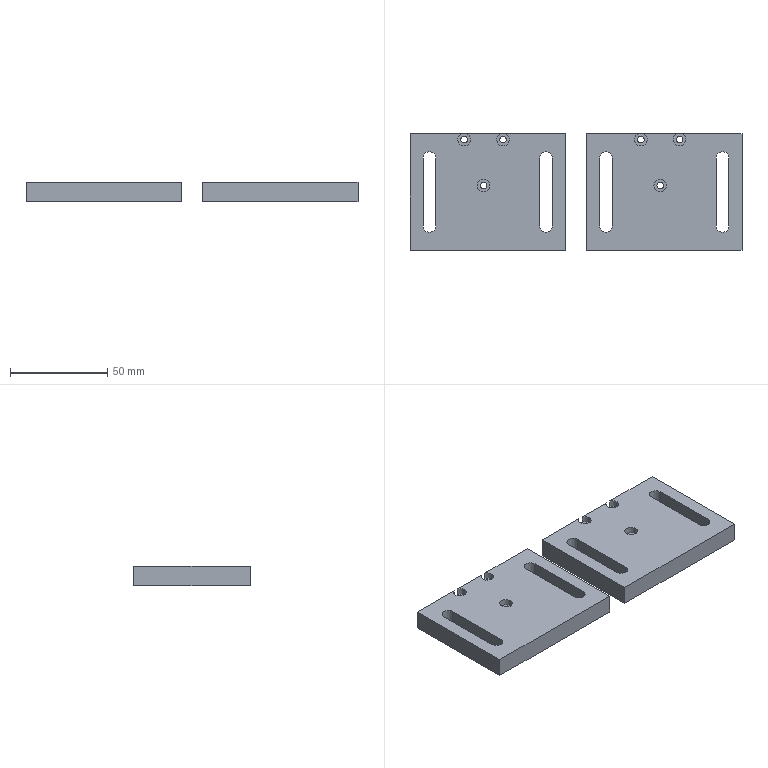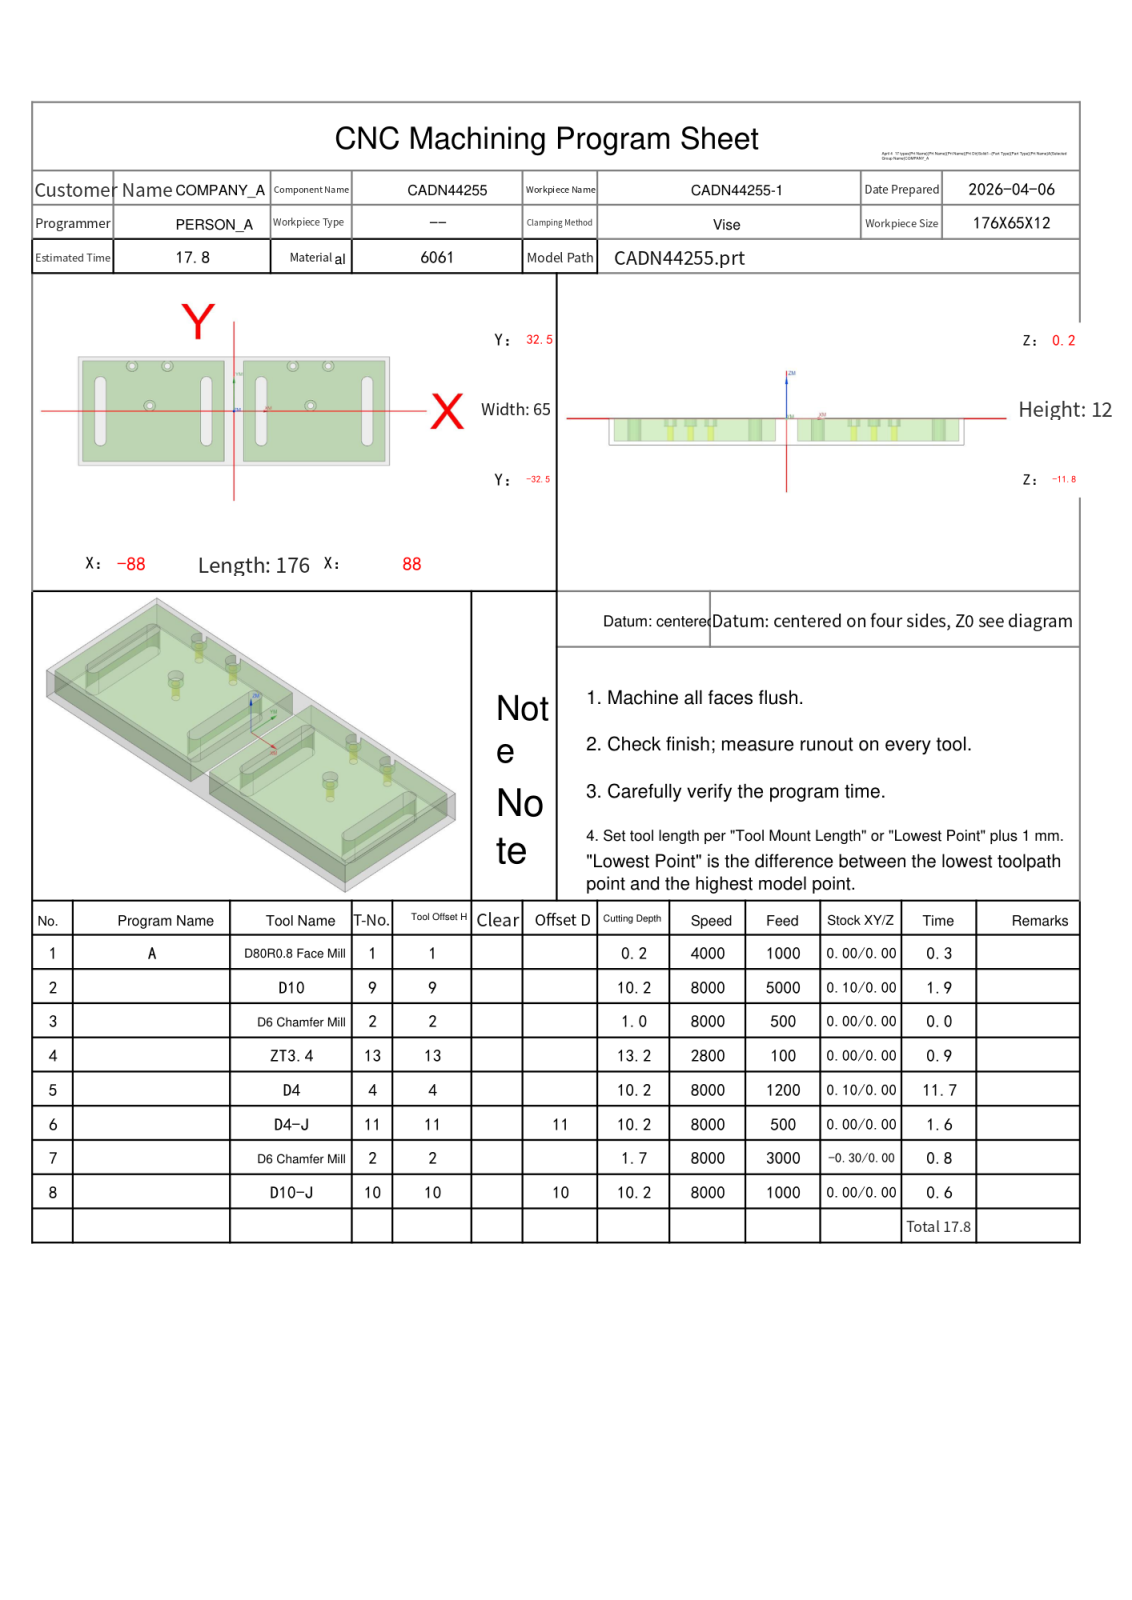NC program | NX | posted by the shop | part box 171 x 60 x 10 mm
Lines 1 to 1630 of 2411, first 1199 of 1628 lines:
%
O0001
(Machine time: 19.33 MIN)
(===Total Tool:7===)
(T1=D80R0.8 Face Mill D=80.  R=0.8  D-  H01 Z=0.    )
(T9=D10     D=10.  R=0.   D-  H09 Z=-10.  )
(T2=D6 Chamfer Mill  D=6.  R=0.  D-  H02 Z=-1.5  )
(T13=ZT3.4  D=3.4  DR_a=118 D-  H13 Z=-13.02)
(T4=D4      D=4.   R=0.   D-  H04 Z=-10.  )
(T11=D4-J   D=4.   R=0.   D11 H11 Z=-10.  )
(T10=D10-J  D=10.  R=0.   D10 H10 Z=-10.  )
G80 G90 G17 G49 G40
G91 G28 Z0
M01
N1 T01 M06
(D80R0.8 Face Mill  D=80. R=0.8 H=01 ce=0.00 di=0.00)
G00 G90 G54 X-130.5 Y0.0 M03 S4000
G43 H01 Z20.
M08
Z2.
G01 Z0.0 F1000.
X-125.5
X125.5
X130.5
Z2.
G00 Z20.
G91 G28 Z0.0
M05
M09
G91 G28 Z0.0
M01
N2 T09 M06
(D10  D=10. R=0. H=09 ce=0.10 di=0.00)
G00 G90 G54 X-45.5 Y-35.1 M03 S8000
G43 H09 Z20.
M08
Z.5
G01 X-85.5 Z.404 F5000.
G02 X-90.6 Y-30. Z.385 I0.0 J5.1
G01 Y30. Z.24
G02 X-85.5 Y35.1 Z.221 I5.1 J0.0
G01 X-5.5 Z.029
G02 X-.4 Y30. Z.01 I0.0 J-5.1
G01 Y-30. Z-.135
G02 X-5.5 Y-35.1 Z-.154 I-5.1 J0.0
G01 X-85.5 Z-.346
G02 X-90.6 Y-30. Z-.365 I0.0 J5.1
G01 Y30. Z-.51
G02 X-85.5 Y35.1 Z-.529 I5.1 J0.0
G01 X-5.5 Z-.721
G02 X-.4 Y30. Z-.74 I0.0 J-5.1
G01 Y-30. Z-.885
G02 X-5.5 Y-35.1 Z-.904 I-5.1 J0.0
G01 X-85.5 Z-1.096
G02 X-90.6 Y-30. Z-1.115 I0.0 J5.1
G01 Y30. Z-1.26
G02 X-85.5 Y35.1 Z-1.279 I5.1 J0.0
G01 X-5.5 Z-1.471
G02 X-.4 Y30. Z-1.49 I0.0 J-5.1
G01 Y-30. Z-1.635
G02 X-5.5 Y-35.1 Z-1.654 I-5.1 J0.0
G01 X-85.5 Z-1.846
G02 X-90.6 Y-30. Z-1.865 I0.0 J5.1
G01 Y30. Z-2.01
G02 X-85.5 Y35.1 Z-2.029 I5.1 J0.0
G01 X-5.5 Z-2.221
G02 X-.4 Y30. Z-2.24 I0.0 J-5.1
G01 Y-30. Z-2.385
G02 X-5.5 Y-35.1 Z-2.404 I-5.1 J0.0
G01 X-85.5 Z-2.596
G02 X-90.6 Y-30. Z-2.615 I0.0 J5.1
G01 Y30. Z-2.76
G02 X-85.5 Y35.1 Z-2.779 I5.1 J0.0
G01 X-5.5 Z-2.971
G02 X-.4 Y30. Z-2.99 I0.0 J-5.1
G01 Y-30. Z-3.135
G02 X-5.5 Y-35.1 Z-3.154 I-5.1 J0.0
G01 X-85.5 Z-3.346
G02 X-90.6 Y-30. Z-3.365 I0.0 J5.1
G01 Y30. Z-3.51
G02 X-85.5 Y35.1 Z-3.529 I5.1 J0.0
G01 X-5.5 Z-3.721
G02 X-.4 Y30. Z-3.74 I0.0 J-5.1
G01 Y-30. Z-3.885
G02 X-5.5 Y-35.1 Z-3.904 I-5.1 J0.0
G01 X-85.5 Z-4.096
G02 X-90.6 Y-30. Z-4.115 I0.0 J5.1
G01 Y30. Z-4.26
G02 X-85.5 Y35.1 Z-4.279 I5.1 J0.0
G01 X-5.5 Z-4.471
G02 X-.4 Y30. Z-4.49 I0.0 J-5.1
G01 Y-30. Z-4.635
G02 X-5.5 Y-35.1 Z-4.654 I-5.1 J0.0
G01 X-85.5 Z-4.846
G02 X-90.6 Y-30. Z-4.865 I0.0 J5.1
G01 Y30. Z-5.01
G02 X-85.5 Y35.1 Z-5.029 I5.1 J0.0
G01 X-5.5 Z-5.221
G02 X-.4 Y30. Z-5.24 I0.0 J-5.1
G01 Y-30. Z-5.385
G02 X-5.5 Y-35.1 Z-5.404 I-5.1 J0.0
G01 X-85.5 Z-5.596
G02 X-90.6 Y-30. Z-5.615 I0.0 J5.1
G01 Y30. Z-5.76
G02 X-85.5 Y35.1 Z-5.779 I5.1 J0.0
G01 X-5.5 Z-5.971
G02 X-.4 Y30. Z-5.99 I0.0 J-5.1
G01 Y-30. Z-6.135
G02 X-5.5 Y-35.1 Z-6.154 I-5.1 J0.0
G01 X-85.5 Z-6.346
G02 X-90.6 Y-30. Z-6.365 I0.0 J5.1
G01 Y30. Z-6.51
G02 X-85.5 Y35.1 Z-6.529 I5.1 J0.0
G01 X-5.5 Z-6.721
G02 X-.4 Y30. Z-6.74 I0.0 J-5.1
G01 Y-30. Z-6.885
G02 X-5.5 Y-35.1 Z-6.904 I-5.1 J0.0
G01 X-85.5 Z-7.096
G02 X-90.6 Y-30. Z-7.115 I0.0 J5.1
G01 Y30. Z-7.26
G02 X-85.5 Y35.1 Z-7.279 I5.1 J0.0
G01 X-5.5 Z-7.471
G02 X-.4 Y30. Z-7.49 I0.0 J-5.1
G01 Y-30. Z-7.635
G02 X-5.5 Y-35.1 Z-7.654 I-5.1 J0.0
G01 X-85.5 Z-7.846
G02 X-90.6 Y-30. Z-7.865 I0.0 J5.1
G01 Y30. Z-8.01
G02 X-85.5 Y35.1 Z-8.029 I5.1 J0.0
G01 X-5.5 Z-8.221
G02 X-.4 Y30. Z-8.24 I0.0 J-5.1
G01 Y-30. Z-8.385
G02 X-5.5 Y-35.1 Z-8.404 I-5.1 J0.0
G01 X-85.5 Z-8.596
G02 X-90.6 Y-30. Z-8.615 I0.0 J5.1
G01 Y30. Z-8.76
G02 X-85.5 Y35.1 Z-8.779 I5.1 J0.0
G01 X-5.5 Z-8.971
G02 X-.4 Y30. Z-8.99 I0.0 J-5.1
G01 Y-30. Z-9.135
G02 X-5.5 Y-35.1 Z-9.154 I-5.1 J0.0
G01 X-85.5 Z-9.346
G02 X-90.6 Y-30. Z-9.365 I0.0 J5.1
G01 Y30. Z-9.51
G02 X-85.5 Y35.1 Z-9.529 I5.1 J0.0
G01 X-5.5 Z-9.721
G02 X-.4 Y30. Z-9.74 I0.0 J-5.1
G01 Y-30. Z-9.885
G02 X-5.5 Y-35.1 Z-9.904 I-5.1 J0.0
G01 X-45.5 Z-10.
X-85.5
G02 X-90.6 Y-30. I0.0 J5.1
G01 Y30.
G02 X-85.5 Y35.1 I5.1 J0.0
G01 X-5.5
G02 X-.4 Y30. I0.0 J-5.1
G01 Y-30.
G02 X-5.5 Y-35.1 I-5.1 J0.0
G01 X-45.5
X-46.
Z-9.
G00 Z20.
X45.5
Z.5
G01 X5.5 Z.404
G02 X.4 Y-30. Z.385 I0.0 J5.1
G01 Y30. Z.24
G02 X5.5 Y35.1 Z.221 I5.1 J0.0
G01 X85.5 Z.029
G02 X90.6 Y30. Z.01 I0.0 J-5.1
G01 Y-30. Z-.135
G02 X85.5 Y-35.1 Z-.154 I-5.1 J0.0
G01 X5.5 Z-.346
G02 X.4 Y-30. Z-.365 I0.0 J5.1
G01 Y30. Z-.51
G02 X5.5 Y35.1 Z-.529 I5.1 J0.0
G01 X85.5 Z-.721
G02 X90.6 Y30. Z-.74 I0.0 J-5.1
G01 Y-30. Z-.885
G02 X85.5 Y-35.1 Z-.904 I-5.1 J0.0
G01 X5.5 Z-1.096
G02 X.4 Y-30. Z-1.115 I0.0 J5.1
G01 Y30. Z-1.26
G02 X5.5 Y35.1 Z-1.279 I5.1 J0.0
G01 X85.5 Z-1.471
G02 X90.6 Y30. Z-1.49 I0.0 J-5.1
G01 Y-30. Z-1.635
G02 X85.5 Y-35.1 Z-1.654 I-5.1 J0.0
G01 X5.5 Z-1.846
G02 X.4 Y-30. Z-1.865 I0.0 J5.1
G01 Y30. Z-2.01
G02 X5.5 Y35.1 Z-2.029 I5.1 J0.0
G01 X85.5 Z-2.221
G02 X90.6 Y30. Z-2.24 I0.0 J-5.1
G01 Y-30. Z-2.385
G02 X85.5 Y-35.1 Z-2.404 I-5.1 J0.0
G01 X5.5 Z-2.596
G02 X.4 Y-30. Z-2.615 I0.0 J5.1
G01 Y30. Z-2.76
G02 X5.5 Y35.1 Z-2.779 I5.1 J0.0
G01 X85.5 Z-2.971
G02 X90.6 Y30. Z-2.99 I0.0 J-5.1
G01 Y-30. Z-3.135
G02 X85.5 Y-35.1 Z-3.154 I-5.1 J0.0
G01 X5.5 Z-3.346
G02 X.4 Y-30. Z-3.365 I0.0 J5.1
G01 Y30. Z-3.51
G02 X5.5 Y35.1 Z-3.529 I5.1 J0.0
G01 X85.5 Z-3.721
G02 X90.6 Y30. Z-3.74 I0.0 J-5.1
G01 Y-30. Z-3.885
G02 X85.5 Y-35.1 Z-3.904 I-5.1 J0.0
G01 X5.5 Z-4.096
G02 X.4 Y-30. Z-4.115 I0.0 J5.1
G01 Y30. Z-4.26
G02 X5.5 Y35.1 Z-4.279 I5.1 J0.0
G01 X85.5 Z-4.471
G02 X90.6 Y30. Z-4.49 I0.0 J-5.1
G01 Y-30. Z-4.635
G02 X85.5 Y-35.1 Z-4.654 I-5.1 J0.0
G01 X5.5 Z-4.846
G02 X.4 Y-30. Z-4.865 I0.0 J5.1
G01 Y30. Z-5.01
G02 X5.5 Y35.1 Z-5.029 I5.1 J0.0
G01 X85.5 Z-5.221
G02 X90.6 Y30. Z-5.24 I0.0 J-5.1
G01 Y-30. Z-5.385
G02 X85.5 Y-35.1 Z-5.404 I-5.1 J0.0
G01 X5.5 Z-5.596
G02 X.4 Y-30. Z-5.615 I0.0 J5.1
G01 Y30. Z-5.76
G02 X5.5 Y35.1 Z-5.779 I5.1 J0.0
G01 X85.5 Z-5.971
G02 X90.6 Y30. Z-5.99 I0.0 J-5.1
G01 Y-30. Z-6.135
G02 X85.5 Y-35.1 Z-6.154 I-5.1 J0.0
G01 X5.5 Z-6.346
G02 X.4 Y-30. Z-6.365 I0.0 J5.1
G01 Y30. Z-6.51
G02 X5.5 Y35.1 Z-6.529 I5.1 J0.0
G01 X85.5 Z-6.721
G02 X90.6 Y30. Z-6.74 I0.0 J-5.1
G01 Y-30. Z-6.885
G02 X85.5 Y-35.1 Z-6.904 I-5.1 J0.0
G01 X5.5 Z-7.096
G02 X.4 Y-30. Z-7.115 I0.0 J5.1
G01 Y30. Z-7.26
G02 X5.5 Y35.1 Z-7.279 I5.1 J0.0
G01 X85.5 Z-7.471
G02 X90.6 Y30. Z-7.49 I0.0 J-5.1
G01 Y-30. Z-7.635
G02 X85.5 Y-35.1 Z-7.654 I-5.1 J0.0
G01 X5.5 Z-7.846
G02 X.4 Y-30. Z-7.865 I0.0 J5.1
G01 Y30. Z-8.01
G02 X5.5 Y35.1 Z-8.029 I5.1 J0.0
G01 X85.5 Z-8.221
G02 X90.6 Y30. Z-8.24 I0.0 J-5.1
G01 Y-30. Z-8.385
G02 X85.5 Y-35.1 Z-8.404 I-5.1 J0.0
G01 X5.5 Z-8.596
G02 X.4 Y-30. Z-8.615 I0.0 J5.1
G01 Y30. Z-8.76
G02 X5.5 Y35.1 Z-8.779 I5.1 J0.0
G01 X85.5 Z-8.971
G02 X90.6 Y30. Z-8.99 I0.0 J-5.1
G01 Y-30. Z-9.135
G02 X85.5 Y-35.1 Z-9.154 I-5.1 J0.0
G01 X5.5 Z-9.346
G02 X.4 Y-30. Z-9.365 I0.0 J5.1
G01 Y30. Z-9.51
G02 X5.5 Y35.1 Z-9.529 I5.1 J0.0
G01 X85.5 Z-9.721
G02 X90.6 Y30. Z-9.74 I0.0 J-5.1
G01 Y-30. Z-9.885
G02 X85.5 Y-35.1 Z-9.904 I-5.1 J0.0
G01 X45.5 Z-10.
X5.5
G02 X.4 Y-30. I0.0 J5.1
G01 Y30.
G02 X5.5 Y35.1 I5.1 J0.0
G01 X85.5
G02 X90.6 Y30. I0.0 J-5.1
G01 Y-30.
G02 X85.5 Y-35.1 I-5.1 J0.0
G01 X45.5
X45.
Z-9.
G00 Z20.
G91 G28 Z0.0
M05
M09
G91 G28 Z0.0
M01
N3 T02 M06
(D6 Chamfer Mill  D=6. R=0. H=02 ce=0.00 di=0.00)
G00 G90 G54 X43.393 Y3.3 M03 S8000
G43 H02 Z20.
M08
G98 G81 X43.393 Y3.3 Z-.8 R1. F500.
X53.393 Y27.
X33.393
X-37.607
X-57.607
X-47.607 Y3.3
G80
G00 Z20.
G91 G28 Z0.0
M05
M09
G91 G28 Z0.0
M01
N4 T13 M06
(ZT3.4 D=3.4 DR_a=118 H=13)
G00 G90 G54 X43.393 Y3.3 M03 S2800
G43 H13 Z20.
M08
G98 G83 X43.393 Y3.3 Z-13.021 R1. F100. Q2.
X53.393 Y27.
X33.393
X-37.607
X-57.607
X-47.607 Y3.3
G80
G00 Z20.
G91 G28 Z0.0
M05
M09
G91 G28 Z0.0
M01
N5 T04 M06
(D4  D=4. R=0. H=04 ce=0.10 di=0.10)
G00 G90 G54 X76.65 Y0.0 M03 S6000
G43 H04 Z20.
M08
Z.5
G01 Y17.5 Z.443 F1200.
G03 X75.5 Y18.65 Z.438 I-1.15 J0.0
X74.58 Y18.19 Z.434 I0.0 J-1.15
X74.35 Y17.5 Z.432 I.92 J-.69
G01 Y-17.5 Z.318
G03 X75.5 Y-18.65 Z.313 I1.15 J0.0
X76.65 Y-17.5 Z.307 I0.0 J1.15
G01 Y17.5 Z.193
G03 X75.5 Y18.65 Z.188 I-1.15 J0.0
X74.58 Y18.19 Z.184 I0.0 J-1.15
X74.35 Y17.5 Z.182 I.92 J-.69
G01 Y-17.5 Z.068
G03 X75.5 Y-18.65 Z.063 I1.15 J0.0
X76.65 Y-17.5 Z.057 I0.0 J1.15
G01 Y17.5 Z-.057
G03 X75.5 Y18.65 Z-.063 I-1.15 J0.0
X74.58 Y18.19 Z-.066 I0.0 J-1.15
X74.35 Y17.5 Z-.068 I.92 J-.69
G01 Y-17.5 Z-.182
G03 X75.5 Y-18.65 Z-.188 I1.15 J0.0
X76.65 Y-17.5 Z-.193 I0.0 J1.15
G01 Y17.5 Z-.307
G03 X75.5 Y18.65 Z-.313 I-1.15 J0.0
X74.58 Y18.19 Z-.316 I0.0 J-1.15
X74.35 Y17.5 Z-.318 I.92 J-.69
G01 Y-17.5 Z-.432
G03 X75.5 Y-18.65 Z-.438 I1.15 J0.0
X76.65 Y-17.5 Z-.443 I0.0 J1.15
G01 Y17.5 Z-.557
G03 X75.5 Y18.65 Z-.563 I-1.15 J0.0
X74.58 Y18.19 Z-.566 I0.0 J-1.15
X74.35 Y17.5 Z-.568 I.92 J-.69
G01 Y-17.5 Z-.682
G03 X75.5 Y-18.65 Z-.688 I1.15 J0.0
X76.65 Y-17.5 Z-.693 I0.0 J1.15
G01 Y17.5 Z-.807
G03 X75.5 Y18.65 Z-.813 I-1.15 J0.0
X74.58 Y18.19 Z-.816 I0.0 J-1.15
X74.35 Y17.5 Z-.818 I.92 J-.69
G01 Y-17.5 Z-.932
G03 X75.5 Y-18.65 Z-.938 I1.15 J0.0
X76.65 Y-17.5 Z-.943 I0.0 J1.15
G01 Y17.5 Z-1.057
G03 X75.5 Y18.65 Z-1.063 I-1.15 J0.0
X74.58 Y18.19 Z-1.066 I0.0 J-1.15
X74.35 Y17.5 Z-1.068 I.92 J-.69
G01 Y-17.5 Z-1.182
G03 X75.5 Y-18.65 Z-1.188 I1.15 J0.0
X76.65 Y-17.5 Z-1.193 I0.0 J1.15
G01 Y17.5 Z-1.307
G03 X75.5 Y18.65 Z-1.313 I-1.15 J0.0
X74.58 Y18.19 Z-1.316 I0.0 J-1.15
X74.35 Y17.5 Z-1.318 I.92 J-.69
G01 Y-17.5 Z-1.432
G03 X75.5 Y-18.65 Z-1.438 I1.15 J0.0
X76.65 Y-17.5 Z-1.443 I0.0 J1.15
G01 Y17.5 Z-1.557
G03 X75.5 Y18.65 Z-1.563 I-1.15 J0.0
X74.58 Y18.19 Z-1.566 I0.0 J-1.15
X74.35 Y17.5 Z-1.568 I.92 J-.69
G01 Y-17.5 Z-1.682
G03 X75.5 Y-18.65 Z-1.688 I1.15 J0.0
X76.65 Y-17.5 Z-1.693 I0.0 J1.15
G01 Y17.5 Z-1.807
G03 X75.5 Y18.65 Z-1.813 I-1.15 J0.0
X74.58 Y18.19 Z-1.816 I0.0 J-1.15
X74.35 Y17.5 Z-1.818 I.92 J-.69
G01 Y-17.5 Z-1.932
G03 X75.5 Y-18.65 Z-1.938 I1.15 J0.0
X76.65 Y-17.5 Z-1.943 I0.0 J1.15
G01 Y17.5 Z-2.057
G03 X75.5 Y18.65 Z-2.063 I-1.15 J0.0
X74.58 Y18.19 Z-2.066 I0.0 J-1.15
X74.35 Y17.5 Z-2.068 I.92 J-.69
G01 Y-17.5 Z-2.182
G03 X75.5 Y-18.65 Z-2.188 I1.15 J0.0
X76.65 Y-17.5 Z-2.193 I0.0 J1.15
G01 Y17.5 Z-2.307
G03 X75.5 Y18.65 Z-2.313 I-1.15 J0.0
X74.58 Y18.19 Z-2.316 I0.0 J-1.15
X74.35 Y17.5 Z-2.318 I.92 J-.69
G01 Y-17.5 Z-2.432
G03 X75.5 Y-18.65 Z-2.438 I1.15 J0.0
X76.65 Y-17.5 Z-2.443 I0.0 J1.15
G01 Y17.5 Z-2.557
G03 X75.5 Y18.65 Z-2.563 I-1.15 J0.0
X74.58 Y18.19 Z-2.566 I0.0 J-1.15
X74.35 Y17.5 Z-2.568 I.92 J-.69
G01 Y-17.5 Z-2.682
G03 X75.5 Y-18.65 Z-2.688 I1.15 J0.0
X76.65 Y-17.5 Z-2.693 I0.0 J1.15
G01 Y17.5 Z-2.807
G03 X75.5 Y18.65 Z-2.813 I-1.15 J0.0
X74.58 Y18.19 Z-2.816 I0.0 J-1.15
X74.35 Y17.5 Z-2.818 I.92 J-.69
G01 Y-17.5 Z-2.932
G03 X75.5 Y-18.65 Z-2.938 I1.15 J0.0
X76.65 Y-17.5 Z-2.943 I0.0 J1.15
G01 Y17.5 Z-3.057
G03 X75.5 Y18.65 Z-3.063 I-1.15 J0.0
X74.58 Y18.19 Z-3.066 I0.0 J-1.15
X74.35 Y17.5 Z-3.068 I.92 J-.69
G01 Y-17.5 Z-3.182
G03 X75.5 Y-18.65 Z-3.188 I1.15 J0.0
X76.65 Y-17.5 Z-3.193 I0.0 J1.15
G01 Y17.5 Z-3.307
G03 X75.5 Y18.65 Z-3.313 I-1.15 J0.0
X74.58 Y18.19 Z-3.316 I0.0 J-1.15
X74.35 Y17.5 Z-3.318 I.92 J-.69
G01 Y-17.5 Z-3.432
G03 X75.5 Y-18.65 Z-3.438 I1.15 J0.0
X76.65 Y-17.5 Z-3.443 I0.0 J1.15
G01 Y17.5 Z-3.557
G03 X75.5 Y18.65 Z-3.563 I-1.15 J0.0
X74.58 Y18.19 Z-3.566 I0.0 J-1.15
X74.35 Y17.5 Z-3.568 I.92 J-.69
G01 Y-17.5 Z-3.682
G03 X75.5 Y-18.65 Z-3.688 I1.15 J0.0
X76.65 Y-17.5 Z-3.693 I0.0 J1.15
G01 Y17.5 Z-3.807
G03 X75.5 Y18.65 Z-3.813 I-1.15 J0.0
X74.58 Y18.19 Z-3.816 I0.0 J-1.15
X74.35 Y17.5 Z-3.818 I.92 J-.69
G01 Y-17.5 Z-3.932
G03 X75.5 Y-18.65 Z-3.938 I1.15 J0.0
X76.65 Y-17.5 Z-3.943 I0.0 J1.15
G01 Y17.5 Z-4.057
G03 X75.5 Y18.65 Z-4.063 I-1.15 J0.0
X74.58 Y18.19 Z-4.066 I0.0 J-1.15
X74.35 Y17.5 Z-4.068 I.92 J-.69
G01 Y-17.5 Z-4.182
G03 X75.5 Y-18.65 Z-4.188 I1.15 J0.0
X76.65 Y-17.5 Z-4.193 I0.0 J1.15
G01 Y17.5 Z-4.307
G03 X75.5 Y18.65 Z-4.313 I-1.15 J0.0
X74.58 Y18.19 Z-4.316 I0.0 J-1.15
X74.35 Y17.5 Z-4.318 I.92 J-.69
G01 Y-17.5 Z-4.432
G03 X75.5 Y-18.65 Z-4.438 I1.15 J0.0
X76.65 Y-17.5 Z-4.443 I0.0 J1.15
G01 Y17.5 Z-4.557
G03 X75.5 Y18.65 Z-4.563 I-1.15 J0.0
X74.58 Y18.19 Z-4.566 I0.0 J-1.15
X74.35 Y17.5 Z-4.568 I.92 J-.69
G01 Y-17.5 Z-4.682
G03 X75.5 Y-18.65 Z-4.688 I1.15 J0.0
X76.65 Y-17.5 Z-4.693 I0.0 J1.15
G01 Y17.5 Z-4.807
G03 X75.5 Y18.65 Z-4.813 I-1.15 J0.0
X74.58 Y18.19 Z-4.816 I0.0 J-1.15
X74.35 Y17.5 Z-4.818 I.92 J-.69
G01 Y-17.5 Z-4.932
G03 X75.5 Y-18.65 Z-4.938 I1.15 J0.0
X76.65 Y-17.5 Z-4.943 I0.0 J1.15
G01 Y17.5 Z-5.057
G03 X75.5 Y18.65 Z-5.063 I-1.15 J0.0
X74.58 Y18.19 Z-5.066 I0.0 J-1.15
X74.35 Y17.5 Z-5.068 I.92 J-.69
G01 Y-17.5 Z-5.182
G03 X75.5 Y-18.65 Z-5.188 I1.15 J0.0
X76.65 Y-17.5 Z-5.193 I0.0 J1.15
G01 Y17.5 Z-5.307
G03 X75.5 Y18.65 Z-5.313 I-1.15 J0.0
X74.58 Y18.19 Z-5.316 I0.0 J-1.15
X74.35 Y17.5 Z-5.318 I.92 J-.69
G01 Y-17.5 Z-5.432
G03 X75.5 Y-18.65 Z-5.438 I1.15 J0.0
X76.65 Y-17.5 Z-5.443 I0.0 J1.15
G01 Y17.5 Z-5.557
G03 X75.5 Y18.65 Z-5.563 I-1.15 J0.0
X74.58 Y18.19 Z-5.566 I0.0 J-1.15
X74.35 Y17.5 Z-5.568 I.92 J-.69
G01 Y-17.5 Z-5.682
G03 X75.5 Y-18.65 Z-5.688 I1.15 J0.0
X76.65 Y-17.5 Z-5.693 I0.0 J1.15
G01 Y17.5 Z-5.807
G03 X75.5 Y18.65 Z-5.813 I-1.15 J0.0
X74.58 Y18.19 Z-5.816 I0.0 J-1.15
X74.35 Y17.5 Z-5.818 I.92 J-.69
G01 Y-17.5 Z-5.932
G03 X75.5 Y-18.65 Z-5.938 I1.15 J0.0
X76.65 Y-17.5 Z-5.943 I0.0 J1.15
G01 Y17.5 Z-6.057
G03 X75.5 Y18.65 Z-6.063 I-1.15 J0.0
X74.58 Y18.19 Z-6.066 I0.0 J-1.15
X74.35 Y17.5 Z-6.068 I.92 J-.69
G01 Y-17.5 Z-6.182
G03 X75.5 Y-18.65 Z-6.188 I1.15 J0.0
X76.65 Y-17.5 Z-6.193 I0.0 J1.15
G01 Y17.5 Z-6.307
G03 X75.5 Y18.65 Z-6.313 I-1.15 J0.0
X74.58 Y18.19 Z-6.316 I0.0 J-1.15
X74.35 Y17.5 Z-6.318 I.92 J-.69
G01 Y-17.5 Z-6.432
G03 X75.5 Y-18.65 Z-6.438 I1.15 J0.0
X76.65 Y-17.5 Z-6.443 I0.0 J1.15
G01 Y17.5 Z-6.557
G03 X75.5 Y18.65 Z-6.563 I-1.15 J0.0
X74.58 Y18.19 Z-6.566 I0.0 J-1.15
X74.35 Y17.5 Z-6.568 I.92 J-.69
G01 Y-17.5 Z-6.682
G03 X75.5 Y-18.65 Z-6.688 I1.15 J0.0
X76.65 Y-17.5 Z-6.693 I0.0 J1.15
G01 Y17.5 Z-6.807
G03 X75.5 Y18.65 Z-6.813 I-1.15 J0.0
X74.58 Y18.19 Z-6.816 I0.0 J-1.15
X74.35 Y17.5 Z-6.818 I.92 J-.69
G01 Y-17.5 Z-6.932
G03 X75.5 Y-18.65 Z-6.938 I1.15 J0.0
X76.65 Y-17.5 Z-6.943 I0.0 J1.15
G01 Y17.5 Z-7.057
G03 X75.5 Y18.65 Z-7.063 I-1.15 J0.0
X74.58 Y18.19 Z-7.066 I0.0 J-1.15
X74.35 Y17.5 Z-7.068 I.92 J-.69
G01 Y-17.5 Z-7.182
G03 X75.5 Y-18.65 Z-7.188 I1.15 J0.0
X76.65 Y-17.5 Z-7.193 I0.0 J1.15
G01 Y17.5 Z-7.307
G03 X75.5 Y18.65 Z-7.313 I-1.15 J0.0
X74.58 Y18.19 Z-7.316 I0.0 J-1.15
X74.35 Y17.5 Z-7.318 I.92 J-.69
G01 Y-17.5 Z-7.432
G03 X75.5 Y-18.65 Z-7.438 I1.15 J0.0
X76.65 Y-17.5 Z-7.443 I0.0 J1.15
G01 Y17.5 Z-7.557
G03 X75.5 Y18.65 Z-7.563 I-1.15 J0.0
X74.58 Y18.19 Z-7.566 I0.0 J-1.15
X74.35 Y17.5 Z-7.568 I.92 J-.69
G01 Y-17.5 Z-7.682
G03 X75.5 Y-18.65 Z-7.688 I1.15 J0.0
X76.65 Y-17.5 Z-7.693 I0.0 J1.15
G01 Y17.5 Z-7.807
G03 X75.5 Y18.65 Z-7.813 I-1.15 J0.0
X74.58 Y18.19 Z-7.816 I0.0 J-1.15
X74.35 Y17.5 Z-7.818 I.92 J-.69
G01 Y-17.5 Z-7.932
G03 X75.5 Y-18.65 Z-7.938 I1.15 J0.0
X76.65 Y-17.5 Z-7.943 I0.0 J1.15
G01 Y17.5 Z-8.057
G03 X75.5 Y18.65 Z-8.063 I-1.15 J0.0
X74.58 Y18.19 Z-8.066 I0.0 J-1.15
X74.35 Y17.5 Z-8.068 I.92 J-.69
G01 Y-17.5 Z-8.182
G03 X75.5 Y-18.65 Z-8.188 I1.15 J0.0
X76.65 Y-17.5 Z-8.193 I0.0 J1.15
G01 Y17.5 Z-8.307
G03 X75.5 Y18.65 Z-8.313 I-1.15 J0.0
X74.58 Y18.19 Z-8.316 I0.0 J-1.15
X74.35 Y17.5 Z-8.318 I.92 J-.69
G01 Y-17.5 Z-8.432
G03 X75.5 Y-18.65 Z-8.438 I1.15 J0.0
X76.65 Y-17.5 Z-8.443 I0.0 J1.15
G01 Y17.5 Z-8.557
G03 X75.5 Y18.65 Z-8.563 I-1.15 J0.0
X74.58 Y18.19 Z-8.566 I0.0 J-1.15
X74.35 Y17.5 Z-8.568 I.92 J-.69
G01 Y-17.5 Z-8.682
G03 X75.5 Y-18.65 Z-8.688 I1.15 J0.0
X76.65 Y-17.5 Z-8.693 I0.0 J1.15
G01 Y17.5 Z-8.807
G03 X75.5 Y18.65 Z-8.813 I-1.15 J0.0
X74.58 Y18.19 Z-8.816 I0.0 J-1.15
X74.35 Y17.5 Z-8.818 I.92 J-.69
G01 Y-17.5 Z-8.932
G03 X75.5 Y-18.65 Z-8.938 I1.15 J0.0
X76.65 Y-17.5 Z-8.943 I0.0 J1.15
G01 Y17.5 Z-9.057
G03 X75.5 Y18.65 Z-9.063 I-1.15 J0.0
X74.58 Y18.19 Z-9.066 I0.0 J-1.15
X74.35 Y17.5 Z-9.068 I.92 J-.69
G01 Y-17.5 Z-9.182
G03 X75.5 Y-18.65 Z-9.188 I1.15 J0.0
X76.65 Y-17.5 Z-9.193 I0.0 J1.15
G01 Y17.5 Z-9.307
G03 X75.5 Y18.65 Z-9.313 I-1.15 J0.0
X74.58 Y18.19 Z-9.316 I0.0 J-1.15
X74.35 Y17.5 Z-9.318 I.92 J-.69
G01 Y-17.5 Z-9.432
G03 X75.5 Y-18.65 Z-9.438 I1.15 J0.0
X76.65 Y-17.5 Z-9.443 I0.0 J1.15
G01 Y17.5 Z-9.557
G03 X75.5 Y18.65 Z-9.563 I-1.15 J0.0
X74.58 Y18.19 Z-9.566 I0.0 J-1.15
X74.35 Y17.5 Z-9.568 I.92 J-.69
G01 Y-17.5 Z-9.682
G03 X75.5 Y-18.65 Z-9.688 I1.15 J0.0
X76.65 Y-17.5 Z-9.693 I0.0 J1.15
G01 Y17.5 Z-9.807
G03 X75.5 Y18.65 Z-9.813 I-1.15 J0.0
X74.58 Y18.19 Z-9.816 I0.0 J-1.15
X74.35 Y17.5 Z-9.818 I.92 J-.69
G01 Y-17.5 Z-9.932
G03 X75.5 Y-18.65 Z-9.938 I1.15 J0.0
X76.65 Y-17.5 Z-9.943 I0.0 J1.15
G01 Y0.0 Z-10.
Y17.5
G03 X75.5 Y18.65 I-1.15 J0.0
X74.35 Y17.5 I0.0 J-1.15
G01 Y-17.5
G03 X75.5 Y-18.65 I1.15 J0.0
X76.65 Y-17.5 I0.0 J1.15
G01 Y0.0
Y.5
Z-9.
G00 Z20.
X16.65 Y0.0
Z.5
G01 Y17.5 Z.443
G03 X15.5 Y18.65 Z.438 I-1.15 J0.0
X14.35 Y17.5 Z.432 I0.0 J-1.15
G01 Y-17.5 Z.318
G03 X15.5 Y-18.65 Z.313 I1.15 J0.0
X16.65 Y-17.5 Z.307 I0.0 J1.15
G01 Y17.5 Z.193
G03 X15.5 Y18.65 Z.188 I-1.15 J0.0
X14.35 Y17.5 Z.182 I0.0 J-1.15
G01 Y-17.5 Z.068
G03 X15.5 Y-18.65 Z.063 I1.15 J0.0
X16.65 Y-17.5 Z.057 I0.0 J1.15
G01 Y17.5 Z-.057
G03 X15.5 Y18.65 Z-.063 I-1.15 J0.0
X14.35 Y17.5 Z-.068 I0.0 J-1.15
G01 Y-17.5 Z-.182
G03 X15.5 Y-18.65 Z-.188 I1.15 J0.0
X16.65 Y-17.5 Z-.193 I0.0 J1.15
G01 Y17.5 Z-.307
G03 X15.5 Y18.65 Z-.313 I-1.15 J0.0
X14.35 Y17.5 Z-.318 I0.0 J-1.15
G01 Y-17.5 Z-.432
G03 X15.5 Y-18.65 Z-.438 I1.15 J0.0
X16.65 Y-17.5 Z-.443 I0.0 J1.15
G01 Y17.5 Z-.557
G03 X15.5 Y18.65 Z-.563 I-1.15 J0.0
X14.35 Y17.5 Z-.568 I0.0 J-1.15
G01 Y-17.5 Z-.682
G03 X15.5 Y-18.65 Z-.688 I1.15 J0.0
X16.65 Y-17.5 Z-.693 I0.0 J1.15
G01 Y17.5 Z-.807
G03 X15.5 Y18.65 Z-.813 I-1.15 J0.0
X14.35 Y17.5 Z-.818 I0.0 J-1.15
G01 Y-17.5 Z-.932
G03 X15.5 Y-18.65 Z-.938 I1.15 J0.0
X16.65 Y-17.5 Z-.943 I0.0 J1.15
G01 Y17.5 Z-1.057
G03 X15.5 Y18.65 Z-1.063 I-1.15 J0.0
X14.35 Y17.5 Z-1.068 I0.0 J-1.15
G01 Y-17.5 Z-1.182
G03 X15.5 Y-18.65 Z-1.188 I1.15 J0.0
X16.65 Y-17.5 Z-1.193 I0.0 J1.15
G01 Y17.5 Z-1.307
G03 X15.5 Y18.65 Z-1.313 I-1.15 J0.0
X14.35 Y17.5 Z-1.318 I0.0 J-1.15
G01 Y-17.5 Z-1.432
G03 X15.5 Y-18.65 Z-1.438 I1.15 J0.0
X16.65 Y-17.5 Z-1.443 I0.0 J1.15
G01 Y17.5 Z-1.557
G03 X15.5 Y18.65 Z-1.563 I-1.15 J0.0
X14.35 Y17.5 Z-1.568 I0.0 J-1.15
G01 Y-17.5 Z-1.682
G03 X15.5 Y-18.65 Z-1.688 I1.15 J0.0
X16.65 Y-17.5 Z-1.693 I0.0 J1.15
G01 Y17.5 Z-1.807
G03 X15.5 Y18.65 Z-1.813 I-1.15 J0.0
X14.35 Y17.5 Z-1.818 I0.0 J-1.15
G01 Y-17.5 Z-1.932
G03 X15.5 Y-18.65 Z-1.938 I1.15 J0.0
X16.65 Y-17.5 Z-1.943 I0.0 J1.15
G01 Y17.5 Z-2.057
G03 X15.5 Y18.65 Z-2.063 I-1.15 J0.0
X14.35 Y17.5 Z-2.068 I0.0 J-1.15
G01 Y-17.5 Z-2.182
G03 X15.5 Y-18.65 Z-2.188 I1.15 J0.0
X16.65 Y-17.5 Z-2.193 I0.0 J1.15
G01 Y17.5 Z-2.307
G03 X15.5 Y18.65 Z-2.313 I-1.15 J0.0
X14.35 Y17.5 Z-2.318 I0.0 J-1.15
G01 Y-17.5 Z-2.432
G03 X15.5 Y-18.65 Z-2.438 I1.15 J0.0
X16.65 Y-17.5 Z-2.443 I0.0 J1.15
G01 Y17.5 Z-2.557
G03 X15.5 Y18.65 Z-2.563 I-1.15 J0.0
X14.35 Y17.5 Z-2.568 I0.0 J-1.15
G01 Y-17.5 Z-2.682
G03 X15.5 Y-18.65 Z-2.688 I1.15 J0.0
X16.65 Y-17.5 Z-2.693 I0.0 J1.15
G01 Y17.5 Z-2.807
G03 X15.5 Y18.65 Z-2.813 I-1.15 J0.0
X14.35 Y17.5 Z-2.818 I0.0 J-1.15
G01 Y-17.5 Z-2.932
G03 X15.5 Y-18.65 Z-2.938 I1.15 J0.0
X16.65 Y-17.5 Z-2.943 I0.0 J1.15
G01 Y17.5 Z-3.057
G03 X15.5 Y18.65 Z-3.063 I-1.15 J0.0
X14.35 Y17.5 Z-3.068 I0.0 J-1.15
G01 Y-17.5 Z-3.182
G03 X15.5 Y-18.65 Z-3.188 I1.15 J0.0
X16.65 Y-17.5 Z-3.193 I0.0 J1.15
G01 Y17.5 Z-3.307
G03 X15.5 Y18.65 Z-3.313 I-1.15 J0.0
X14.35 Y17.5 Z-3.318 I0.0 J-1.15
G01 Y-17.5 Z-3.432
G03 X15.5 Y-18.65 Z-3.438 I1.15 J0.0
X16.65 Y-17.5 Z-3.443 I0.0 J1.15
G01 Y17.5 Z-3.557
G03 X15.5 Y18.65 Z-3.563 I-1.15 J0.0
X14.35 Y17.5 Z-3.568 I0.0 J-1.15
G01 Y-17.5 Z-3.682
G03 X15.5 Y-18.65 Z-3.688 I1.15 J0.0
X16.65 Y-17.5 Z-3.693 I0.0 J1.15
G01 Y17.5 Z-3.807
G03 X15.5 Y18.65 Z-3.813 I-1.15 J0.0
X14.35 Y17.5 Z-3.818 I0.0 J-1.15
G01 Y-17.5 Z-3.932
G03 X15.5 Y-18.65 Z-3.938 I1.15 J0.0
X16.65 Y-17.5 Z-3.943 I0.0 J1.15
G01 Y17.5 Z-4.057
G03 X15.5 Y18.65 Z-4.063 I-1.15 J0.0
X14.35 Y17.5 Z-4.068 I0.0 J-1.15
G01 Y-17.5 Z-4.182
G03 X15.5 Y-18.65 Z-4.188 I1.15 J0.0
X16.65 Y-17.5 Z-4.193 I0.0 J1.15
G01 Y17.5 Z-4.307
G03 X15.5 Y18.65 Z-4.313 I-1.15 J0.0
X14.35 Y17.5 Z-4.318 I0.0 J-1.15
G01 Y-17.5 Z-4.432
G03 X15.5 Y-18.65 Z-4.438 I1.15 J0.0
X16.65 Y-17.5 Z-4.443 I0.0 J1.15
G01 Y17.5 Z-4.557
G03 X15.5 Y18.65 Z-4.563 I-1.15 J0.0
X14.35 Y17.5 Z-4.568 I0.0 J-1.15
G01 Y-17.5 Z-4.682
G03 X15.5 Y-18.65 Z-4.688 I1.15 J0.0
X16.65 Y-17.5 Z-4.693 I0.0 J1.15
G01 Y17.5 Z-4.807
G03 X15.5 Y18.65 Z-4.813 I-1.15 J0.0
X14.35 Y17.5 Z-4.818 I0.0 J-1.15
G01 Y-17.5 Z-4.932
G03 X15.5 Y-18.65 Z-4.938 I1.15 J0.0
X16.65 Y-17.5 Z-4.943 I0.0 J1.15
G01 Y17.5 Z-5.057
G03 X15.5 Y18.65 Z-5.063 I-1.15 J0.0
X14.35 Y17.5 Z-5.068 I0.0 J-1.15
G01 Y-17.5 Z-5.182
G03 X15.5 Y-18.65 Z-5.188 I1.15 J0.0
X16.65 Y-17.5 Z-5.193 I0.0 J1.15
G01 Y17.5 Z-5.307
G03 X15.5 Y18.65 Z-5.313 I-1.15 J0.0
X14.35 Y17.5 Z-5.318 I0.0 J-1.15
G01 Y-17.5 Z-5.432
G03 X15.5 Y-18.65 Z-5.438 I1.15 J0.0
X16.65 Y-17.5 Z-5.443 I0.0 J1.15
G01 Y17.5 Z-5.557
G03 X15.5 Y18.65 Z-5.563 I-1.15 J0.0
X14.35 Y17.5 Z-5.568 I0.0 J-1.15
G01 Y-17.5 Z-5.682
G03 X15.5 Y-18.65 Z-5.688 I1.15 J0.0
X16.65 Y-17.5 Z-5.693 I0.0 J1.15
G01 Y17.5 Z-5.807
G03 X15.5 Y18.65 Z-5.813 I-1.15 J0.0
X14.35 Y17.5 Z-5.818 I0.0 J-1.15
G01 Y-17.5 Z-5.932
G03 X15.5 Y-18.65 Z-5.938 I1.15 J0.0
X16.65 Y-17.5 Z-5.943 I0.0 J1.15
G01 Y17.5 Z-6.057
G03 X15.5 Y18.65 Z-6.063 I-1.15 J0.0
X14.35 Y17.5 Z-6.068 I0.0 J-1.15
G01 Y-17.5 Z-6.182
G03 X15.5 Y-18.65 Z-6.188 I1.15 J0.0
X16.65 Y-17.5 Z-6.193 I0.0 J1.15
G01 Y17.5 Z-6.307
G03 X15.5 Y18.65 Z-6.313 I-1.15 J0.0
X14.35 Y17.5 Z-6.318 I0.0 J-1.15
G01 Y-17.5 Z-6.432
G03 X15.5 Y-18.65 Z-6.438 I1.15 J0.0
X16.65 Y-17.5 Z-6.443 I0.0 J1.15
G01 Y17.5 Z-6.557
G03 X15.5 Y18.65 Z-6.563 I-1.15 J0.0
X14.35 Y17.5 Z-6.568 I0.0 J-1.15
G01 Y-17.5 Z-6.682
G03 X15.5 Y-18.65 Z-6.688 I1.15 J0.0
X16.65 Y-17.5 Z-6.693 I0.0 J1.15
G01 Y17.5 Z-6.807
G03 X15.5 Y18.65 Z-6.813 I-1.15 J0.0
X14.35 Y17.5 Z-6.818 I0.0 J-1.15
G01 Y-17.5 Z-6.932
G03 X15.5 Y-18.65 Z-6.938 I1.15 J0.0
X16.65 Y-17.5 Z-6.943 I0.0 J1.15
G01 Y17.5 Z-7.057
G03 X15.5 Y18.65 Z-7.063 I-1.15 J0.0
X14.35 Y17.5 Z-7.068 I0.0 J-1.15
G01 Y-17.5 Z-7.182
G03 X15.5 Y-18.65 Z-7.188 I1.15 J0.0
X16.65 Y-17.5 Z-7.193 I0.0 J1.15
G01 Y17.5 Z-7.307
G03 X15.5 Y18.65 Z-7.313 I-1.15 J0.0
X14.35 Y17.5 Z-7.318 I0.0 J-1.15
G01 Y-17.5 Z-7.432
G03 X15.5 Y-18.65 Z-7.438 I1.15 J0.0
X16.65 Y-17.5 Z-7.443 I0.0 J1.15
G01 Y17.5 Z-7.557
G03 X15.5 Y18.65 Z-7.563 I-1.15 J0.0
X14.35 Y17.5 Z-7.568 I0.0 J-1.15
G01 Y-17.5 Z-7.682
G03 X15.5 Y-18.65 Z-7.688 I1.15 J0.0
X16.65 Y-17.5 Z-7.693 I0.0 J1.15
G01 Y17.5 Z-7.807
G03 X15.5 Y18.65 Z-7.813 I-1.15 J0.0
X14.35 Y17.5 Z-7.818 I0.0 J-1.15
G01 Y-17.5 Z-7.932
G03 X15.5 Y-18.65 Z-7.938 I1.15 J0.0
X16.65 Y-17.5 Z-7.943 I0.0 J1.15
G01 Y17.5 Z-8.057
G03 X15.5 Y18.65 Z-8.063 I-1.15 J0.0
X14.35 Y17.5 Z-8.068 I0.0 J-1.15
G01 Y-17.5 Z-8.182
G03 X15.5 Y-18.65 Z-8.188 I1.15 J0.0
X16.65 Y-17.5 Z-8.193 I0.0 J1.15
G01 Y17.5 Z-8.307
G03 X15.5 Y18.65 Z-8.313 I-1.15 J0.0
X14.35 Y17.5 Z-8.318 I0.0 J-1.15
G01 Y-17.5 Z-8.432
G03 X15.5 Y-18.65 Z-8.438 I1.15 J0.0
X16.65 Y-17.5 Z-8.443 I0.0 J1.15
G01 Y17.5 Z-8.557
G03 X15.5 Y18.65 Z-8.563 I-1.15 J0.0
X14.35 Y17.5 Z-8.568 I0.0 J-1.15
G01 Y-17.5 Z-8.682
G03 X15.5 Y-18.65 Z-8.688 I1.15 J0.0
X16.65 Y-17.5 Z-8.693 I0.0 J1.15
G01 Y17.5 Z-8.807
G03 X15.5 Y18.65 Z-8.813 I-1.15 J0.0
X14.35 Y17.5 Z-8.818 I0.0 J-1.15
G01 Y-17.5 Z-8.932
G03 X15.5 Y-18.65 Z-8.938 I1.15 J0.0
X16.65 Y-17.5 Z-8.943 I0.0 J1.15
G01 Y17.5 Z-9.057
G03 X15.5 Y18.65 Z-9.063 I-1.15 J0.0
X14.35 Y17.5 Z-9.068 I0.0 J-1.15
G01 Y-17.5 Z-9.182
G03 X15.5 Y-18.65 Z-9.188 I1.15 J0.0
X16.65 Y-17.5 Z-9.193 I0.0 J1.15
G01 Y17.5 Z-9.307
G03 X15.5 Y18.65 Z-9.313 I-1.15 J0.0
X14.35 Y17.5 Z-9.318 I0.0 J-1.15
G01 Y-17.5 Z-9.432
G03 X15.5 Y-18.65 Z-9.438 I1.15 J0.0
X16.65 Y-17.5 Z-9.443 I0.0 J1.15
G01 Y17.5 Z-9.557
G03 X15.5 Y18.65 Z-9.563 I-1.15 J0.0
X14.35 Y17.5 Z-9.568 I0.0 J-1.15
G01 Y-17.5 Z-9.682
G03 X15.5 Y-18.65 Z-9.688 I1.15 J0.0
X16.65 Y-17.5 Z-9.693 I0.0 J1.15
G01 Y17.5 Z-9.807
G03 X15.5 Y18.65 Z-9.813 I-1.15 J0.0
X14.35 Y17.5 Z-9.818 I0.0 J-1.15
G01 Y-17.5 Z-9.932
G03 X15.5 Y-18.65 Z-9.938 I1.15 J0.0
X16.65 Y-17.5 Z-9.943 I0.0 J1.15
G01 Y0.0 Z-10.
Y17.5
G03 X15.5 Y18.65 I-1.15 J0.0
X14.35 Y17.5 I0.0 J-1.15
G01 Y-17.5
G03 X15.5 Y-18.65 I1.15 J0.0
X16.65 Y-17.5 I0.0 J1.15
G01 Y0.0
Y.5
Z-9.
G00 Z20.
X-14.35 Y0.0
Z.5
G01 Y17.5 Z.443
G03 X-15.5 Y18.65 Z.438 I-1.15 J0.0
X-16.65 Y17.5 Z.432 I0.0 J-1.15
G01 Y-17.5 Z.318
G03 X-15.5 Y-18.65 Z.313 I1.15 J0.0
X-14.35 Y-17.5 Z.307 I0.0 J1.15
G01 Y17.5 Z.193
G03 X-15.5 Y18.65 Z.188 I-1.15 J0.0
X-16.65 Y17.5 Z.182 I0.0 J-1.15
G01 Y-17.5 Z.068
G03 X-15.5 Y-18.65 Z.063 I1.15 J0.0
X-14.35 Y-17.5 Z.057 I0.0 J1.15
G01 Y17.5 Z-.057
G03 X-15.5 Y18.65 Z-.063 I-1.15 J0.0
X-16.65 Y17.5 Z-.068 I0.0 J-1.15
G01 Y-17.5 Z-.182
G03 X-15.5 Y-18.65 Z-.188 I1.15 J0.0
X-14.35 Y-17.5 Z-.193 I0.0 J1.15
G01 Y17.5 Z-.307
G03 X-15.5 Y18.65 Z-.313 I-1.15 J0.0
X-16.65 Y17.5 Z-.318 I0.0 J-1.15
G01 Y-17.5 Z-.432
G03 X-15.5 Y-18.65 Z-.438 I1.15 J0.0
X-14.35 Y-17.5 Z-.443 I0.0 J1.15
G01 Y17.5 Z-.557
G03 X-15.5 Y18.65 Z-.563 I-1.15 J0.0
X-16.65 Y17.5 Z-.568 I0.0 J-1.15
G01 Y-17.5 Z-.682
G03 X-15.5 Y-18.65 Z-.688 I1.15 J0.0
X-14.35 Y-17.5 Z-.693 I0.0 J1.15
G01 Y17.5 Z-.807
G03 X-15.5 Y18.65 Z-.813 I-1.15 J0.0
X-16.65 Y17.5 Z-.818 I0.0 J-1.15
G01 Y-17.5 Z-.932
G03 X-15.5 Y-18.65 Z-.938 I1.15 J0.0
X-14.35 Y-17.5 Z-.943 I0.0 J1.15
G01 Y17.5 Z-1.057
G03 X-15.5 Y18.65 Z-1.063 I-1.15 J0.0
X-16.65 Y17.5 Z-1.068 I0.0 J-1.15
G01 Y-17.5 Z-1.182
G03 X-15.5 Y-18.65 Z-1.188 I1.15 J0.0
X-14.35 Y-17.5 Z-1.193 I0.0 J1.15
G01 Y17.5 Z-1.307
G03 X-15.5 Y18.65 Z-1.313 I-1.15 J0.0
X-16.65 Y17.5 Z-1.318 I0.0 J-1.15
G01 Y-17.5 Z-1.432
G03 X-15.5 Y-18.65 Z-1.438 I1.15 J0.0
X-14.35 Y-17.5 Z-1.443 I0.0 J1.15
G01 Y17.5 Z-1.557
G03 X-15.5 Y18.65 Z-1.563 I-1.15 J0.0
X-16.65 Y17.5 Z-1.568 I0.0 J-1.15
G01 Y-17.5 Z-1.682
G03 X-15.5 Y-18.65 Z-1.688 I1.15 J0.0
X-14.35 Y-17.5 Z-1.693 I0.0 J1.15
G01 Y17.5 Z-1.807
G03 X-15.5 Y18.65 Z-1.813 I-1.15 J0.0
X-16.65 Y17.5 Z-1.818 I0.0 J-1.15
G01 Y-17.5 Z-1.932
G03 X-15.5 Y-18.65 Z-1.938 I1.15 J0.0
X-14.35 Y-17.5 Z-1.943 I0.0 J1.15
G01 Y17.5 Z-2.057
G03 X-15.5 Y18.65 Z-2.063 I-1.15 J0.0
X-16.65 Y17.5 Z-2.068 I0.0 J-1.15
G01 Y-17.5 Z-2.182
G03 X-15.5 Y-18.65 Z-2.188 I1.15 J0.0
X-14.35 Y-17.5 Z-2.193 I0.0 J1.15
G01 Y17.5 Z-2.307
G03 X-15.5 Y18.65 Z-2.313 I-1.15 J0.0
X-16.65 Y17.5 Z-2.318 I0.0 J-1.15
G01 Y-17.5 Z-2.432
G03 X-15.5 Y-18.65 Z-2.438 I1.15 J0.0
X-14.35 Y-17.5 Z-2.443 I0.0 J1.15
G01 Y17.5 Z-2.557
G03 X-15.5 Y18.65 Z-2.563 I-1.15 J0.0
X-16.65 Y17.5 Z-2.568 I0.0 J-1.15
G01 Y-17.5 Z-2.682
G03 X-15.5 Y-18.65 Z-2.688 I1.15 J0.0
X-14.35 Y-17.5 Z-2.693 I0.0 J1.15
G01 Y17.5 Z-2.807
G03 X-15.5 Y18.65 Z-2.813 I-1.15 J0.0
X-16.65 Y17.5 Z-2.818 I0.0 J-1.15
G01 Y-17.5 Z-2.932
G03 X-15.5 Y-18.65 Z-2.938 I1.15 J0.0
X-14.35 Y-17.5 Z-2.943 I0.0 J1.15
G01 Y17.5 Z-3.057
G03 X-15.5 Y18.65 Z-3.063 I-1.15 J0.0
X-16.65 Y17.5 Z-3.068 I0.0 J-1.15
G01 Y-17.5 Z-3.182
G03 X-15.5 Y-18.65 Z-3.188 I1.15 J0.0
X-14.35 Y-17.5 Z-3.193 I0.0 J1.15
G01 Y17.5 Z-3.307
G03 X-15.5 Y18.65 Z-3.313 I-1.15 J0.0
X-16.65 Y17.5 Z-3.318 I0.0 J-1.15
G01 Y-17.5 Z-3.432
G03 X-15.5 Y-18.65 Z-3.438 I1.15 J0.0
X-14.35 Y-17.5 Z-3.443 I0.0 J1.15
G01 Y17.5 Z-3.557
G03 X-15.5 Y18.65 Z-3.563 I-1.15 J0.0
X-16.65 Y17.5 Z-3.568 I0.0 J-1.15
G01 Y-17.5 Z-3.682
G03 X-15.5 Y-18.65 Z-3.688 I1.15 J0.0
X-14.35 Y-17.5 Z-3.693 I0.0 J1.15
G01 Y17.5 Z-3.807
G03 X-15.5 Y18.65 Z-3.813 I-1.15 J0.0
X-16.65 Y17.5 Z-3.818 I0.0 J-1.15
G01 Y-17.5 Z-3.932
G03 X-15.5 Y-18.65 Z-3.938 I1.15 J0.0
X-14.35 Y-17.5 Z-3.943 I0.0 J1.15
G01 Y17.5 Z-4.057
G03 X-15.5 Y18.65 Z-4.063 I-1.15 J0.0
X-16.65 Y17.5 Z-4.068 I0.0 J-1.15
G01 Y-17.5 Z-4.182
G03 X-15.5 Y-18.65 Z-4.188 I1.15 J0.0
X-14.35 Y-17.5 Z-4.193 I0.0 J1.15
G01 Y17.5 Z-4.307
G03 X-15.5 Y18.65 Z-4.313 I-1.15 J0.0
X-16.65 Y17.5 Z-4.318 I0.0 J-1.15
G01 Y-17.5 Z-4.432
G03 X-15.5 Y-18.65 Z-4.438 I1.15 J0.0
X-14.35 Y-17.5 Z-4.443 I0.0 J1.15
G01 Y17.5 Z-4.557
G03 X-15.5 Y18.65 Z-4.563 I-1.15 J0.0
X-16.65 Y17.5 Z-4.568 I0.0 J-1.15
G01 Y-17.5 Z-4.682
G03 X-15.5 Y-18.65 Z-4.688 I1.15 J0.0
X-14.35 Y-17.5 Z-4.693 I0.0 J1.15
G01 Y17.5 Z-4.807
G03 X-15.5 Y18.65 Z-4.813 I-1.15 J0.0
X-16.65 Y17.5 Z-4.818 I0.0 J-1.15
G01 Y-17.5 Z-4.932
G03 X-15.5 Y-18.65 Z-4.938 I1.15 J0.0
X-14.35 Y-17.5 Z-4.943 I0.0 J1.15
G01 Y17.5 Z-5.057
G03 X-15.5 Y18.65 Z-5.063 I-1.15 J0.0
X-16.65 Y17.5 Z-5.068 I0.0 J-1.15
G01 Y-17.5 Z-5.182
G03 X-15.5 Y-18.65 Z-5.188 I1.15 J0.0
X-14.35 Y-17.5 Z-5.193 I0.0 J1.15
G01 Y17.5 Z-5.307
G03 X-15.5 Y18.65 Z-5.313 I-1.15 J0.0
X-16.65 Y17.5 Z-5.318 I0.0 J-1.15
G01 Y-17.5 Z-5.432
G03 X-15.5 Y-18.65 Z-5.438 I1.15 J0.0
X-14.35 Y-17.5 Z-5.443 I0.0 J1.15
G01 Y17.5 Z-5.557
G03 X-15.5 Y18.65 Z-5.563 I-1.15 J0.0
X-16.65 Y17.5 Z-5.568 I0.0 J-1.15
G01 Y-17.5 Z-5.682
G03 X-15.5 Y-18.65 Z-5.688 I1.15 J0.0
X-14.35 Y-17.5 Z-5.693 I0.0 J1.15
G01 Y17.5 Z-5.807
G03 X-15.5 Y18.65 Z-5.813 I-1.15 J0.0
X-16.65 Y17.5 Z-5.818 I0.0 J-1.15
G01 Y-17.5 Z-5.932
G03 X-15.5 Y-18.65 Z-5.938 I1.15 J0.0
X-14.35 Y-17.5 Z-5.943 I0.0 J1.15
G01 Y17.5 Z-6.057
G03 X-15.5 Y18.65 Z-6.063 I-1.15 J0.0
X-16.65 Y17.5 Z-6.068 I0.0 J-1.15
G01 Y-17.5 Z-6.182
G03 X-15.5 Y-18.65 Z-6.188 I1.15 J0.0
X-14.35 Y-17.5 Z-6.193 I0.0 J1.15
G01 Y17.5 Z-6.307
G03 X-15.5 Y18.65 Z-6.313 I-1.15 J0.0
X-16.65 Y17.5 Z-6.318 I0.0 J-1.15
G01 Y-17.5 Z-6.432
G03 X-15.5 Y-18.65 Z-6.438 I1.15 J0.0
X-14.35 Y-17.5 Z-6.443 I0.0 J1.15
G01 Y17.5 Z-6.557
G03 X-15.5 Y18.65 Z-6.563 I-1.15 J0.0
X-16.65 Y17.5 Z-6.568 I0.0 J-1.15
G01 Y-17.5 Z-6.682
G03 X-15.5 Y-18.65 Z-6.688 I1.15 J0.0
X-14.35 Y-17.5 Z-6.693 I0.0 J1.15
G01 Y17.5 Z-6.807
G03 X-15.5 Y18.65 Z-6.813 I-1.15 J0.0
X-16.65 Y17.5 Z-6.818 I0.0 J-1.15
G01 Y-17.5 Z-6.932
G03 X-15.5 Y-18.65 Z-6.938 I1.15 J0.0
X-14.35 Y-17.5 Z-6.943 I0.0 J1.15
G01 Y17.5 Z-7.057
G03 X-15.5 Y18.65 Z-7.063 I-1.15 J0.0
X-16.65 Y17.5 Z-7.068 I0.0 J-1.15
G01 Y-17.5 Z-7.182
G03 X-15.5 Y-18.65 Z-7.188 I1.15 J0.0
X-14.35 Y-17.5 Z-7.193 I0.0 J1.15
G01 Y17.5 Z-7.307
G03 X-15.5 Y18.65 Z-7.313 I-1.15 J0.0
X-16.65 Y17.5 Z-7.318 I0.0 J-1.15
G01 Y-17.5 Z-7.432
G03 X-15.5 Y-18.65 Z-7.438 I1.15 J0.0
X-14.35 Y-17.5 Z-7.443 I0.0 J1.15
G01 Y17.5 Z-7.557
G03 X-15.5 Y18.65 Z-7.563 I-1.15 J0.0
X-16.65 Y17.5 Z-7.568 I0.0 J-1.15
G01 Y-17.5 Z-7.682
G03 X-15.5 Y-18.65 Z-7.688 I1.15 J0.0
X-14.35 Y-17.5 Z-7.693 I0.0 J1.15
G01 Y17.5 Z-7.807
G03 X-15.5 Y18.65 Z-7.813 I-1.15 J0.0
X-16.65 Y17.5 Z-7.818 I0.0 J-1.15
G01 Y-17.5 Z-7.932
G03 X-15.5 Y-18.65 Z-7.938 I1.15 J0.0
X-14.35 Y-17.5 Z-7.943 I0.0 J1.15
G01 Y17.5 Z-8.057
G03 X-15.5 Y18.65 Z-8.063 I-1.15 J0.0
X-16.65 Y17.5 Z-8.068 I0.0 J-1.15
G01 Y-17.5 Z-8.182
G03 X-15.5 Y-18.65 Z-8.188 I1.15 J0.0
X-14.35 Y-17.5 Z-8.193 I0.0 J1.15
G01 Y17.5 Z-8.307
G03 X-15.5 Y18.65 Z-8.313 I-1.15 J0.0
X-16.65 Y17.5 Z-8.318 I0.0 J-1.15
G01 Y-17.5 Z-8.432
G03 X-15.5 Y-18.65 Z-8.438 I1.15 J0.0
X-14.35 Y-17.5 Z-8.443 I0.0 J1.15
G01 Y17.5 Z-8.557
G03 X-15.5 Y18.65 Z-8.563 I-1.15 J0.0
X-16.65 Y17.5 Z-8.568 I0.0 J-1.15
G01 Y-17.5 Z-8.682
G03 X-15.5 Y-18.65 Z-8.688 I1.15 J0.0
X-14.35 Y-17.5 Z-8.693 I0.0 J1.15
G01 Y17.5 Z-8.807
G03 X-15.5 Y18.65 Z-8.813 I-1.15 J0.0
X-16.65 Y17.5 Z-8.818 I0.0 J-1.15
G01 Y-17.5 Z-8.932
G03 X-15.5 Y-18.65 Z-8.938 I1.15 J0.0
X-14.35 Y-17.5 Z-8.943 I0.0 J1.15
G01 Y17.5 Z-9.057
G03 X-15.5 Y18.65 Z-9.063 I-1.15 J0.0
X-16.65 Y17.5 Z-9.068 I0.0 J-1.15
G01 Y-17.5 Z-9.182
G03 X-15.5 Y-18.65 Z-9.188 I1.15 J0.0
X-14.35 Y-17.5 Z-9.193 I0.0 J1.15
G01 Y17.5 Z-9.307
G03 X-15.5 Y18.65 Z-9.313 I-1.15 J0.0
X-16.65 Y17.5 Z-9.318 I0.0 J-1.15
G01 Y-17.5 Z-9.432
G03 X-15.5 Y-18.65 Z-9.438 I1.15 J0.0
X-14.35 Y-17.5 Z-9.443 I0.0 J1.15
G01 Y17.5 Z-9.557
G03 X-15.5 Y18.65 Z-9.563 I-1.15 J0.0
X-16.65 Y17.5 Z-9.568 I0.0 J-1.15
G01 Y-17.5 Z-9.682
G03 X-15.5 Y-18.65 Z-9.688 I1.15 J0.0
X-14.35 Y-17.5 Z-9.693 I0.0 J1.15
G01 Y17.5 Z-9.807
G03 X-15.5 Y18.65 Z-9.813 I-1.15 J0.0
X-16.65 Y17.5 Z-9.818 I0.0 J-1.15
G01 Y-17.5 Z-9.932
G03 X-15.5 Y-18.65 Z-9.938 I1.15 J0.0
X-14.35 Y-17.5 Z-9.943 I0.0 J1.15
G01 Y0.0 Z-10.
Y17.5
G03 X-15.5 Y18.65 I-1.15 J0.0
X-16.65 Y17.5 I0.0 J-1.15
G01 Y-17.5
G03 X-15.5 Y-18.65 I1.15 J0.0
X-14.35 Y-17.5 I0.0 J1.15
G01 Y0.0
Y.5
Z-9.
G00 Z20.
X-76.65 Y0.0
Z.5
G01 Y-17.5 Z.443
G03 X-76.19 Y-18.42 Z.44 I1.15 J0.0
X-75.5 Y-18.65 Z.438 I.69 J.92
X-74.35 Y-17.5 Z.432 I0.0 J1.15
G01 Y17.5 Z.318
G03 X-75.5 Y18.65 Z.313 I-1.15 J0.0
X-76.65 Y17.5 Z.307 I0.0 J-1.15
G01 Y-17.5 Z.193
G03 X-76.19 Y-18.42 Z.19 I1.15 J0.0
X-75.5 Y-18.65 Z.188 I.69 J.92
X-74.35 Y-17.5 Z.182 I0.0 J1.15
G01 Y17.5 Z.068
G03 X-75.5 Y18.65 Z.063 I-1.15 J0.0
X-76.65 Y17.5 Z.057 I0.0 J-1.15
G01 Y-17.5 Z-.057
G03 X-76.19 Y-18.42 Z-.06 I1.15 J0.0
X-75.5 Y-18.65 Z-.063 I.69 J.92
X-74.35 Y-17.5 Z-.068 I0.0 J1.15
G01 Y17.5 Z-.182
G03 X-75.5 Y18.65 Z-.188 I-1.15 J0.0
X-76.65 Y17.5 Z-.193 I0.0 J-1.15
G01 Y-17.5 Z-.307
G03 X-76.19 Y-18.42 Z-.31 I1.15 J0.0
X-75.5 Y-18.65 Z-.313 I.69 J.92
X-74.35 Y-17.5 Z-.318 I0.0 J1.15
G01 Y17.5 Z-.432